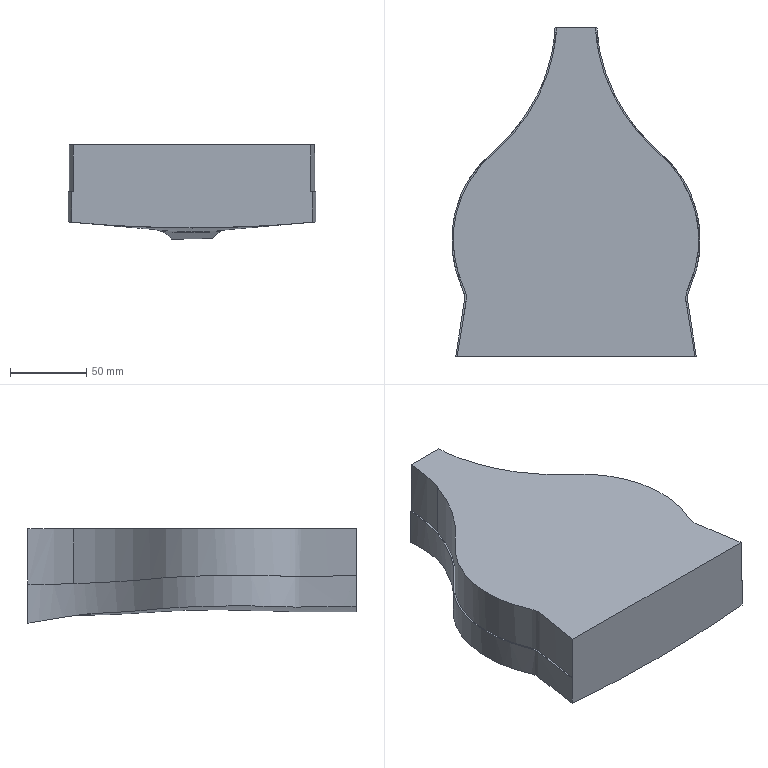Part | NX | features solid 2 | 1 solid | 21 faces | box 162.73 x 214.9 x 61.803 mm | volume 1298843 mm3 | spline 15 | plane 6